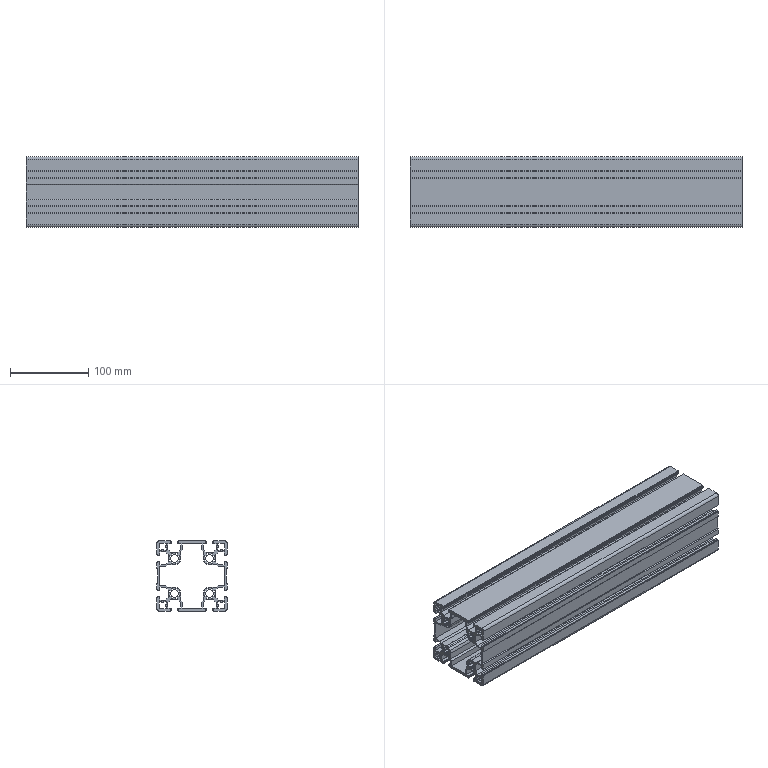Part | STEP file | 001-010-Waste column profile_default<machined> | 1 solid | 406 faces | box 425 x 90 x 90 mm | volume 830601 mm3 | plane 362 | cylinder 44 | commonest cylinder face diameters 10 x36 6.76 x4 16 x4